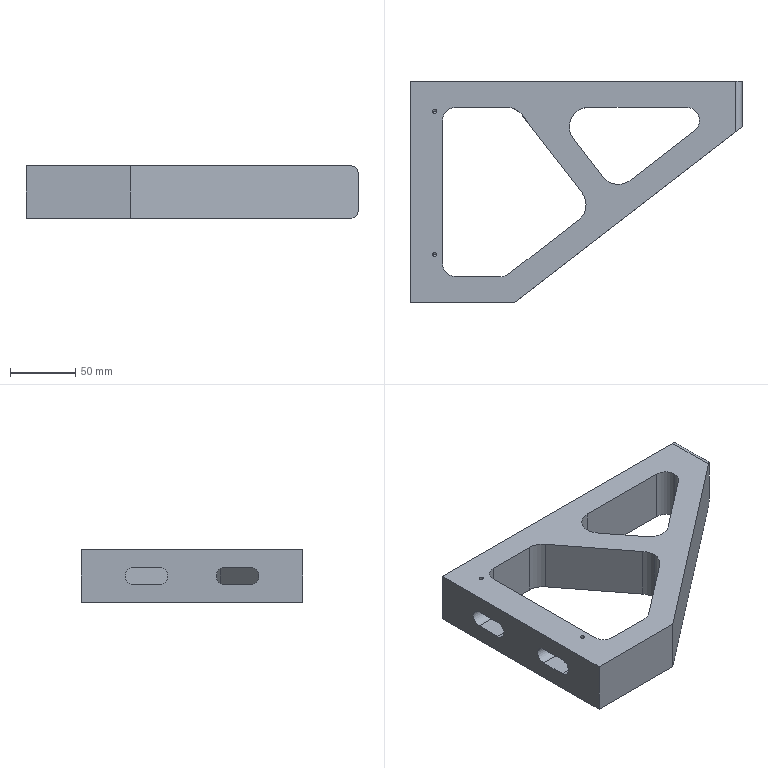Part | NX | features BREP 1 | 1 solid | 70 faces | box 255 x 170 x 40 mm | volume 644245 mm3 | cylinder 34 | plane 20 | cone 16 | commonest cylinder face diameters 3.3 x8 4.2 x6 20 x5 30 x5 5 x4 13 x4